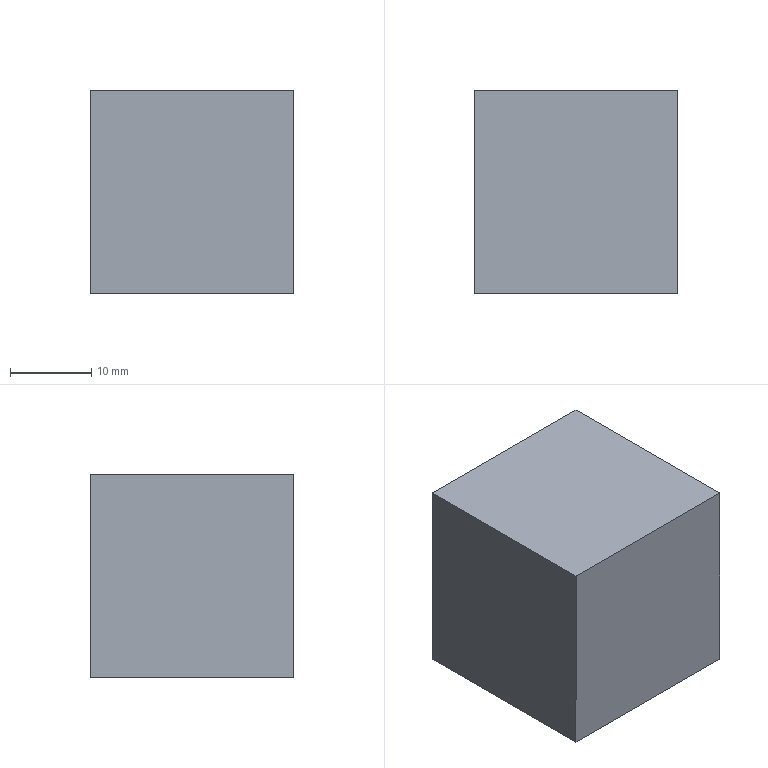Part | SolidWorks | features Extrusion 1 | 1 solid | 6 faces | box 25 x 25 x 25 mm | volume 15625 mm3 | plane 6
STEP:
#1=CARTESIAN_POINT('',(12.5,0.,12.5));
#2=VERTEX_POINT('',#1);
#3=CARTESIAN_POINT('',(12.5,0.,-12.5));
#4=VERTEX_POINT('',#3);
#5=CARTESIAN_POINT('',(12.5,0.,-12.5));
#6=DIRECTION('',(0.,0.,-1.));
#7=VECTOR('',#6,1000.);
#8=LINE('',#5,#7);
#9=EDGE_CURVE('',#2,#4,#8,.T.);
#10=ORIENTED_EDGE('',*,*,#9,.T.);
#11=CARTESIAN_POINT('',(12.5,25.,-12.5));
#12=VERTEX_POINT('',#11);
#13=CARTESIAN_POINT('',(12.5,25.,-12.5));
#14=DIRECTION('',(0.,-1.,0.));
#15=VECTOR('',#14,1000.);
#16=LINE('',#13,#15);
#17=EDGE_CURVE('',#12,#4,#16,.T.);
#18=ORIENTED_EDGE('',*,*,#17,.F.);
#19=CARTESIAN_POINT('',(12.5,25.,12.5));
#20=VERTEX_POINT('',#19);
#21=CARTESIAN_POINT('',(12.5,25.,-12.5));
#22=DIRECTION('',(0.,0.,-1.));
#23=VECTOR('',#22,1000.);
#24=LINE('',#21,#23);
#25=EDGE_CURVE('',#20,#12,#24,.T.);
#26=ORIENTED_EDGE('',*,*,#25,.F.);
#27=CARTESIAN_POINT('',(12.5,25.,12.5));
#28=DIRECTION('',(0.,-1.,0.));
#29=VECTOR('',#28,1000.);
#30=LINE('',#27,#29);
#31=EDGE_CURVE('',#20,#2,#30,.T.);
#32=ORIENTED_EDGE('',*,*,#31,.T.);
#33=EDGE_LOOP('',(#10,#18,#26,#32));
#34=FACE_OUTER_BOUND('',#33,.T.);
#35=CARTESIAN_POINT('',(12.5,25.,-12.5));
#36=DIRECTION('',(-1.,0.,0.));
#37=DIRECTION('',(0.,0.,1.));
#38=AXIS2_PLACEMENT_3D('',#35,#36,#37);
#39=PLANE('',#38);
#40=ADVANCED_FACE('',(#34),#39,.F.);
#41=CARTESIAN_POINT('',(-12.5,0.,-12.5));
#42=VERTEX_POINT('',#41);
#43=CARTESIAN_POINT('',(-12.5,0.,-12.5));
#44=DIRECTION('',(-1.,0.,0.));
#45=VECTOR('',#44,1000.);
#46=LINE('',#43,#45);
#47=EDGE_CURVE('',#4,#42,#46,.T.);
#48=ORIENTED_EDGE('',*,*,#47,.T.);
#49=CARTESIAN_POINT('',(-12.5,25.,-12.5));
#50=VERTEX_POINT('',#49);
#51=CARTESIAN_POINT('',(-12.5,25.,-12.5));
#52=DIRECTION('',(0.,-1.,0.));
#53=VECTOR('',#52,1000.);
#54=LINE('',#51,#53);
#55=EDGE_CURVE('',#50,#42,#54,.T.);
#56=ORIENTED_EDGE('',*,*,#55,.F.);
#57=CARTESIAN_POINT('',(-12.5,25.,-12.5));
#58=DIRECTION('',(-1.,0.,0.));
#59=VECTOR('',#58,1000.);
#60=LINE('',#57,#59);
#61=EDGE_CURVE('',#12,#50,#60,.T.);
#62=ORIENTED_EDGE('',*,*,#61,.F.);
#63=ORIENTED_EDGE('',*,*,#17,.T.);
#64=EDGE_LOOP('',(#48,#56,#62,#63));
#65=FACE_OUTER_BOUND('',#64,.T.);
#66=CARTESIAN_POINT('',(-12.5,25.,-12.5));
#67=DIRECTION('',(0.,0.,1.));
#68=DIRECTION('',(1.,0.,0.));
#69=AXIS2_PLACEMENT_3D('',#66,#67,#68);
#70=PLANE('',#69);
#71=ADVANCED_FACE('',(#65),#70,.F.);
#72=CARTESIAN_POINT('',(-12.5,0.,12.5));
#73=VERTEX_POINT('',#72);
#74=CARTESIAN_POINT('',(-12.5,0.,-12.5));
#75=DIRECTION('',(0.,0.,1.));
#76=VECTOR('',#75,1000.);
#77=LINE('',#74,#76);
#78=EDGE_CURVE('',#42,#73,#77,.T.);
#79=ORIENTED_EDGE('',*,*,#78,.T.);
#80=CARTESIAN_POINT('',(-12.5,25.,12.5));
#81=VERTEX_POINT('',#80);
#82=CARTESIAN_POINT('',(-12.5,25.,12.5));
#83=DIRECTION('',(0.,-1.,0.));
#84=VECTOR('',#83,1000.);
#85=LINE('',#82,#84);
#86=EDGE_CURVE('',#81,#73,#85,.T.);
#87=ORIENTED_EDGE('',*,*,#86,.F.);
#88=CARTESIAN_POINT('',(-12.5,25.,-12.5));
#89=DIRECTION('',(0.,0.,1.));
#90=VECTOR('',#89,1000.);
#91=LINE('',#88,#90);
#92=EDGE_CURVE('',#50,#81,#91,.T.);
#93=ORIENTED_EDGE('',*,*,#92,.F.);
#94=ORIENTED_EDGE('',*,*,#55,.T.);
#95=EDGE_LOOP('',(#79,#87,#93,#94));
#96=FACE_OUTER_BOUND('',#95,.T.);
#97=CARTESIAN_POINT('',(-12.5,25.,-12.5));
#98=DIRECTION('',(1.,0.,0.));
#99=DIRECTION('',(0.,0.,-1.));
#100=AXIS2_PLACEMENT_3D('',#97,#98,#99);
#101=PLANE('',#100);
#102=ADVANCED_FACE('',(#96),#101,.F.);
#103=CARTESIAN_POINT('',(-12.5,0.,12.5));
#104=DIRECTION('',(1.,0.,0.));
#105=VECTOR('',#104,1000.);
#106=LINE('',#103,#105);
#107=EDGE_CURVE('',#73,#2,#106,.T.);
#108=ORIENTED_EDGE('',*,*,#107,.T.);
#109=ORIENTED_EDGE('',*,*,#31,.F.);
#110=CARTESIAN_POINT('',(-12.5,25.,12.5));
#111=DIRECTION('',(1.,0.,0.));
#112=VECTOR('',#111,1000.);
#113=LINE('',#110,#112);
#114=EDGE_CURVE('',#81,#20,#113,.T.);
#115=ORIENTED_EDGE('',*,*,#114,.F.);
#116=ORIENTED_EDGE('',*,*,#86,.T.);
#117=EDGE_LOOP('',(#108,#109,#115,#116));
#118=FACE_OUTER_BOUND('',#117,.T.);
#119=CARTESIAN_POINT('',(-12.5,25.,12.5));
#120=DIRECTION('',(0.,0.,-1.));
#121=DIRECTION('',(-1.,0.,0.));
#122=AXIS2_PLACEMENT_3D('',#119,#120,#121);
#123=PLANE('',#122);
#124=ADVANCED_FACE('',(#118),#123,.F.);
#125=ORIENTED_EDGE('',*,*,#25,.T.);
#126=ORIENTED_EDGE('',*,*,#61,.T.);
#127=ORIENTED_EDGE('',*,*,#92,.T.);
#128=ORIENTED_EDGE('',*,*,#114,.T.);
#129=EDGE_LOOP('',(#125,#126,#127,#128));
#130=FACE_OUTER_BOUND('',#129,.T.);
#131=CARTESIAN_POINT('',(0.,25.,0.));
#132=DIRECTION('',(0.,1.,0.));
#133=DIRECTION('',(0.,0.,1.));
#134=AXIS2_PLACEMENT_3D('',#131,#132,#133);
#135=PLANE('',#134);
#136=ADVANCED_FACE('',(#130),#135,.T.);
#137=ORIENTED_EDGE('',*,*,#9,.F.);
#138=ORIENTED_EDGE('',*,*,#107,.F.);
#139=ORIENTED_EDGE('',*,*,#78,.F.);
#140=ORIENTED_EDGE('',*,*,#47,.F.);
#141=EDGE_LOOP('',(#137,#138,#139,#140));
#142=FACE_OUTER_BOUND('',#141,.T.);
#143=CARTESIAN_POINT('',(0.,0.,0.));
#144=DIRECTION('',(0.,1.,0.));
#145=DIRECTION('',(0.,0.,1.));
#146=AXIS2_PLACEMENT_3D('',#143,#144,#145);
#147=PLANE('',#146);
#148=ADVANCED_FACE('',(#142),#147,.F.);
#149=CLOSED_SHELL('',(#40,#71,#102,#124,#136,#148));
#150=MANIFOLD_SOLID_BREP('',#149);
#151=CARTESIAN_POINT('',(0.,0.,0.));
#152=DIRECTION('',(0.,0.,1.));
#153=DIRECTION('',(1.,0.,0.));
#154=AXIS2_PLACEMENT_3D('',#151,#152,#153);
#155=(LENGTH_UNIT()NAMED_UNIT(*)SI_UNIT(.MILLI.,.METRE.));
#156=UNCERTAINTY_MEASURE_WITH_UNIT(LENGTH_MEASURE(0.00001),#155,'','');
#157=(NAMED_UNIT(*)PLANE_ANGLE_UNIT()SI_UNIT($,.RADIAN.));
#158=(NAMED_UNIT(*)SI_UNIT($,.STERADIAN.)SOLID_ANGLE_UNIT());
#159=(GEOMETRIC_REPRESENTATION_CONTEXT(3)GLOBAL_UNCERTAINTY_ASSIGNED_CONTEXT((#156))GLOBAL_UNIT_ASSIGNED_CONTEXT((#155,#157,#158))REPRESENTATION_CONTEXT('',''));
#160=ADVANCED_BREP_SHAPE_REPRESENTATION('',(#150,#154),#159);